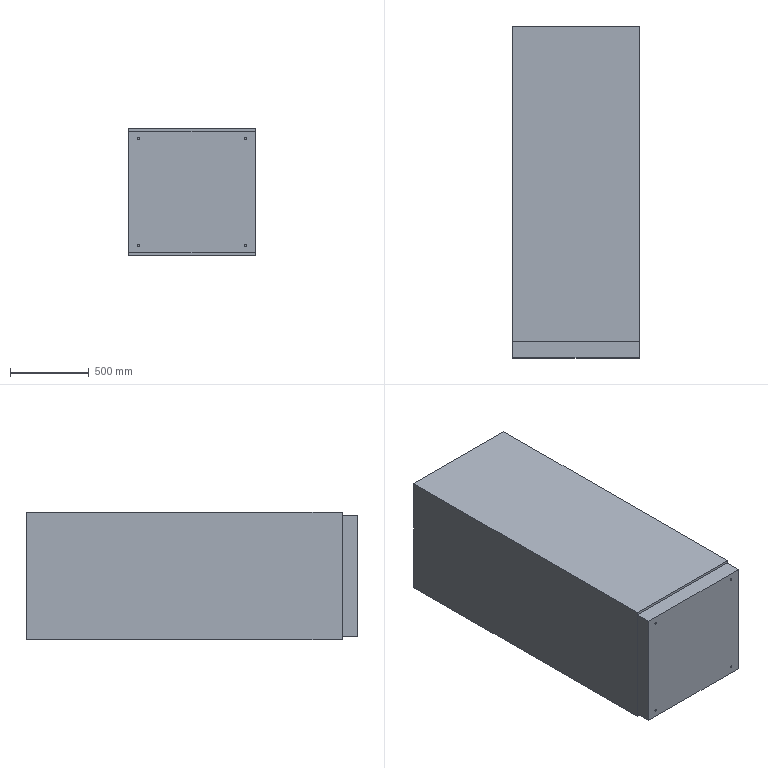Part | STEP file | PLC cabinet | 1 solid | 125 faces | box 806 x 2100 x 805 mm | volume 1358956656 mm3 | plane 72 | spline 45 | cylinder 8 | commonest cylinder face diameters 14 x8